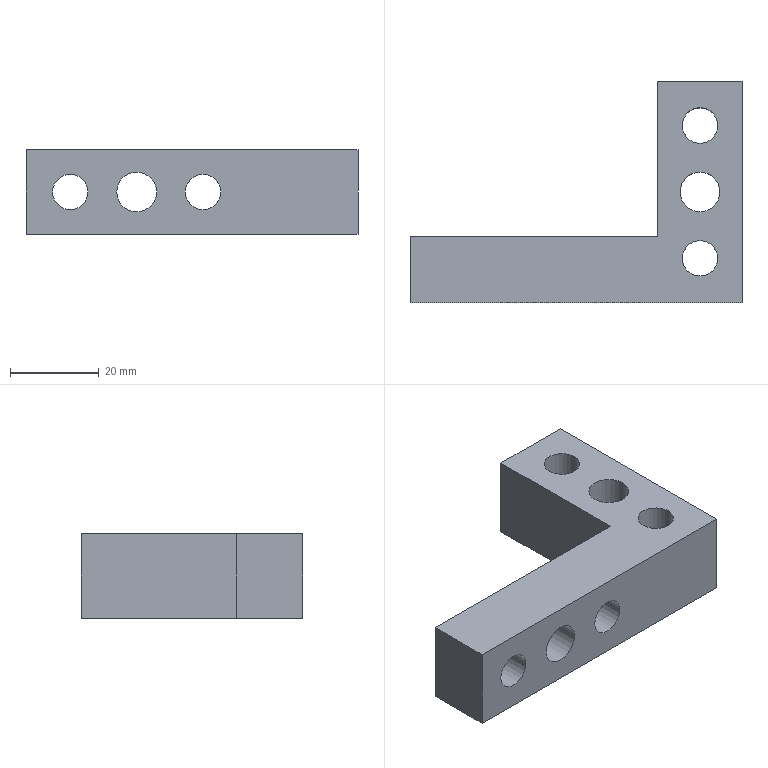Part | SolidWorks | features Extrusion 1, ICE 1 | 1 solid | 20 faces | box 75 x 50 x 19 mm | volume 28429 mm3 | cylinder 12 | plane 8 | commonest cylinder face diameters 8 x8 9 x4
STEP:
#1=CARTESIAN_POINT('',(14.,0.,9.5));
#2=VERTEX_POINT('',#1);
#3=CARTESIAN_POINT('',(6.,0.,9.5));
#4=VERTEX_POINT('',#3);
#5=CARTESIAN_POINT('',(10.,0.,9.5));
#6=DIRECTION('',(0.,1.,0.));
#7=DIRECTION('',(0.,0.,1.));
#8=AXIS2_PLACEMENT_3D('',#5,#6,#7);
#9=CIRCLE('',#8,4.);
#10=EDGE_CURVE('',#2,#4,#9,.T.);
#11=ORIENTED_EDGE('',*,*,#10,.F.);
#12=CARTESIAN_POINT('',(14.,15.,9.5));
#13=VERTEX_POINT('',#12);
#14=CARTESIAN_POINT('',(14.,-4.,9.5));
#15=DIRECTION('',(0.,1.,0.));
#16=VECTOR('',#15,1000.);
#17=LINE('',#14,#16);
#18=EDGE_CURVE('',#2,#13,#17,.T.);
#19=ORIENTED_EDGE('',*,*,#18,.T.);
#20=CARTESIAN_POINT('',(6.,15.,9.5));
#21=VERTEX_POINT('',#20);
#22=CARTESIAN_POINT('',(10.,15.,9.5));
#23=DIRECTION('',(0.,1.,0.));
#24=DIRECTION('',(-1.,0.,0.));
#25=AXIS2_PLACEMENT_3D('',#22,#23,#24);
#26=CIRCLE('',#25,4.);
#27=EDGE_CURVE('',#13,#21,#26,.T.);
#28=ORIENTED_EDGE('',*,*,#27,.T.);
#29=CARTESIAN_POINT('',(6.,-4.,9.5));
#30=DIRECTION('',(0.,1.,0.));
#31=VECTOR('',#30,1000.);
#32=LINE('',#29,#31);
#33=EDGE_CURVE('',#4,#21,#32,.T.);
#34=ORIENTED_EDGE('',*,*,#33,.F.);
#35=EDGE_LOOP('',(#11,#19,#28,#34));
#36=FACE_OUTER_BOUND('',#35,.T.);
#37=CARTESIAN_POINT('',(10.,-4.,9.5));
#38=DIRECTION('',(0.,1.,0.));
#39=DIRECTION('',(-1.,0.,0.));
#40=AXIS2_PLACEMENT_3D('',#37,#38,#39);
#41=CYLINDRICAL_SURFACE('',#40,4.);
#42=ADVANCED_FACE('',(#36),#41,.F.);
#43=CARTESIAN_POINT('',(29.5,0.,9.5));
#44=VERTEX_POINT('',#43);
#45=CARTESIAN_POINT('',(20.5,0.,9.5));
#46=VERTEX_POINT('',#45);
#47=CARTESIAN_POINT('',(25.,0.,9.5));
#48=DIRECTION('',(0.,1.,0.));
#49=DIRECTION('',(0.,0.,1.));
#50=AXIS2_PLACEMENT_3D('',#47,#48,#49);
#51=CIRCLE('',#50,4.5);
#52=EDGE_CURVE('',#44,#46,#51,.T.);
#53=ORIENTED_EDGE('',*,*,#52,.F.);
#54=CARTESIAN_POINT('',(29.5,15.,9.5));
#55=VERTEX_POINT('',#54);
#56=CARTESIAN_POINT('',(29.5,-4.,9.5));
#57=DIRECTION('',(0.,1.,0.));
#58=VECTOR('',#57,1000.);
#59=LINE('',#56,#58);
#60=EDGE_CURVE('',#44,#55,#59,.T.);
#61=ORIENTED_EDGE('',*,*,#60,.T.);
#62=CARTESIAN_POINT('',(20.5,15.,9.5));
#63=VERTEX_POINT('',#62);
#64=CARTESIAN_POINT('',(25.,15.,9.5));
#65=DIRECTION('',(0.,1.,0.));
#66=DIRECTION('',(-1.,0.,0.));
#67=AXIS2_PLACEMENT_3D('',#64,#65,#66);
#68=CIRCLE('',#67,4.5);
#69=EDGE_CURVE('',#55,#63,#68,.T.);
#70=ORIENTED_EDGE('',*,*,#69,.T.);
#71=CARTESIAN_POINT('',(20.5,-4.,9.5));
#72=DIRECTION('',(0.,1.,0.));
#73=VECTOR('',#72,1000.);
#74=LINE('',#71,#73);
#75=EDGE_CURVE('',#46,#63,#74,.T.);
#76=ORIENTED_EDGE('',*,*,#75,.F.);
#77=EDGE_LOOP('',(#53,#61,#70,#76));
#78=FACE_OUTER_BOUND('',#77,.T.);
#79=CARTESIAN_POINT('',(25.,-4.,9.5));
#80=DIRECTION('',(0.,1.,0.));
#81=DIRECTION('',(-1.,0.,0.));
#82=AXIS2_PLACEMENT_3D('',#79,#80,#81);
#83=CYLINDRICAL_SURFACE('',#82,4.5);
#84=ADVANCED_FACE('',(#78),#83,.F.);
#85=CARTESIAN_POINT('',(44.,0.,9.5));
#86=VERTEX_POINT('',#85);
#87=CARTESIAN_POINT('',(36.,0.,9.5));
#88=VERTEX_POINT('',#87);
#89=CARTESIAN_POINT('',(40.,0.,9.5));
#90=DIRECTION('',(0.,1.,0.));
#91=DIRECTION('',(0.,0.,1.));
#92=AXIS2_PLACEMENT_3D('',#89,#90,#91);
#93=CIRCLE('',#92,4.);
#94=EDGE_CURVE('',#86,#88,#93,.T.);
#95=ORIENTED_EDGE('',*,*,#94,.F.);
#96=CARTESIAN_POINT('',(44.,15.,9.5));
#97=VERTEX_POINT('',#96);
#98=CARTESIAN_POINT('',(44.,-4.,9.5));
#99=DIRECTION('',(0.,1.,0.));
#100=VECTOR('',#99,1000.);
#101=LINE('',#98,#100);
#102=EDGE_CURVE('',#86,#97,#101,.T.);
#103=ORIENTED_EDGE('',*,*,#102,.T.);
#104=CARTESIAN_POINT('',(36.,15.,9.5));
#105=VERTEX_POINT('',#104);
#106=CARTESIAN_POINT('',(40.,15.,9.5));
#107=DIRECTION('',(0.,1.,0.));
#108=DIRECTION('',(-1.,0.,0.));
#109=AXIS2_PLACEMENT_3D('',#106,#107,#108);
#110=CIRCLE('',#109,4.);
#111=EDGE_CURVE('',#97,#105,#110,.T.);
#112=ORIENTED_EDGE('',*,*,#111,.T.);
#113=CARTESIAN_POINT('',(36.,-4.,9.5));
#114=DIRECTION('',(0.,1.,0.));
#115=VECTOR('',#114,1000.);
#116=LINE('',#113,#115);
#117=EDGE_CURVE('',#88,#105,#116,.T.);
#118=ORIENTED_EDGE('',*,*,#117,.F.);
#119=EDGE_LOOP('',(#95,#103,#112,#118));
#120=FACE_OUTER_BOUND('',#119,.T.);
#121=CARTESIAN_POINT('',(40.,-4.,9.5));
#122=DIRECTION('',(0.,1.,0.));
#123=DIRECTION('',(-1.,0.,0.));
#124=AXIS2_PLACEMENT_3D('',#121,#122,#123);
#125=CYLINDRICAL_SURFACE('',#124,4.);
#126=ADVANCED_FACE('',(#120),#125,.F.);
#127=CARTESIAN_POINT('',(61.5,40.,19.));
#128=VERTEX_POINT('',#127);
#129=CARTESIAN_POINT('',(69.5,40.,19.));
#130=VERTEX_POINT('',#129);
#131=CARTESIAN_POINT('',(65.5,40.,19.));
#132=DIRECTION('',(0.,0.,1.));
#133=DIRECTION('',(1.,0.,0.));
#134=AXIS2_PLACEMENT_3D('',#131,#132,#133);
#135=CIRCLE('',#134,4.);
#136=EDGE_CURVE('',#128,#130,#135,.T.);
#137=ORIENTED_EDGE('',*,*,#136,.T.);
#138=CARTESIAN_POINT('',(69.5,40.,0.));
#139=VERTEX_POINT('',#138);
#140=CARTESIAN_POINT('',(69.5,40.,19.));
#141=DIRECTION('',(0.,0.,-1.));
#142=VECTOR('',#141,1000.);
#143=LINE('',#140,#142);
#144=EDGE_CURVE('',#130,#139,#143,.T.);
#145=ORIENTED_EDGE('',*,*,#144,.T.);
#146=CARTESIAN_POINT('',(61.5,40.,0.));
#147=VERTEX_POINT('',#146);
#148=CARTESIAN_POINT('',(65.5,40.,0.));
#149=DIRECTION('',(0.,0.,1.));
#150=DIRECTION('',(1.,0.,0.));
#151=AXIS2_PLACEMENT_3D('',#148,#149,#150);
#152=CIRCLE('',#151,4.);
#153=EDGE_CURVE('',#147,#139,#152,.T.);
#154=ORIENTED_EDGE('',*,*,#153,.F.);
#155=CARTESIAN_POINT('',(61.5,40.,19.));
#156=DIRECTION('',(0.,0.,-1.));
#157=VECTOR('',#156,1000.);
#158=LINE('',#155,#157);
#159=EDGE_CURVE('',#128,#147,#158,.T.);
#160=ORIENTED_EDGE('',*,*,#159,.F.);
#161=EDGE_LOOP('',(#137,#145,#154,#160));
#162=FACE_OUTER_BOUND('',#161,.T.);
#163=CARTESIAN_POINT('',(65.5,40.,19.));
#164=DIRECTION('',(0.,0.,-1.));
#165=DIRECTION('',(-1.,0.,0.));
#166=AXIS2_PLACEMENT_3D('',#163,#164,#165);
#167=CYLINDRICAL_SURFACE('',#166,4.);
#168=ADVANCED_FACE('',(#162),#167,.F.);
#169=CARTESIAN_POINT('',(61.,25.,19.));
#170=VERTEX_POINT('',#169);
#171=CARTESIAN_POINT('',(70.,25.,19.));
#172=VERTEX_POINT('',#171);
#173=CARTESIAN_POINT('',(65.5,25.,19.));
#174=DIRECTION('',(0.,0.,1.));
#175=DIRECTION('',(1.,0.,0.));
#176=AXIS2_PLACEMENT_3D('',#173,#174,#175);
#177=CIRCLE('',#176,4.5);
#178=EDGE_CURVE('',#170,#172,#177,.T.);
#179=ORIENTED_EDGE('',*,*,#178,.T.);
#180=CARTESIAN_POINT('',(70.,25.,0.));
#181=VERTEX_POINT('',#180);
#182=CARTESIAN_POINT('',(70.,25.,19.));
#183=DIRECTION('',(0.,0.,-1.));
#184=VECTOR('',#183,1000.);
#185=LINE('',#182,#184);
#186=EDGE_CURVE('',#172,#181,#185,.T.);
#187=ORIENTED_EDGE('',*,*,#186,.T.);
#188=CARTESIAN_POINT('',(61.,25.,0.));
#189=VERTEX_POINT('',#188);
#190=CARTESIAN_POINT('',(65.5,25.,0.));
#191=DIRECTION('',(0.,0.,1.));
#192=DIRECTION('',(1.,0.,0.));
#193=AXIS2_PLACEMENT_3D('',#190,#191,#192);
#194=CIRCLE('',#193,4.5);
#195=EDGE_CURVE('',#189,#181,#194,.T.);
#196=ORIENTED_EDGE('',*,*,#195,.F.);
#197=CARTESIAN_POINT('',(61.,25.,19.));
#198=DIRECTION('',(0.,0.,-1.));
#199=VECTOR('',#198,1000.);
#200=LINE('',#197,#199);
#201=EDGE_CURVE('',#170,#189,#200,.T.);
#202=ORIENTED_EDGE('',*,*,#201,.F.);
#203=EDGE_LOOP('',(#179,#187,#196,#202));
#204=FACE_OUTER_BOUND('',#203,.T.);
#205=CARTESIAN_POINT('',(65.5,25.,19.));
#206=DIRECTION('',(0.,0.,-1.));
#207=DIRECTION('',(-1.,0.,0.));
#208=AXIS2_PLACEMENT_3D('',#205,#206,#207);
#209=CYLINDRICAL_SURFACE('',#208,4.5);
#210=ADVANCED_FACE('',(#204),#209,.F.);
#211=CARTESIAN_POINT('',(61.5,10.,19.));
#212=VERTEX_POINT('',#211);
#213=CARTESIAN_POINT('',(69.5,10.,19.));
#214=VERTEX_POINT('',#213);
#215=CARTESIAN_POINT('',(65.5,10.,19.));
#216=DIRECTION('',(0.,0.,1.));
#217=DIRECTION('',(1.,0.,0.));
#218=AXIS2_PLACEMENT_3D('',#215,#216,#217);
#219=CIRCLE('',#218,4.);
#220=EDGE_CURVE('',#212,#214,#219,.T.);
#221=ORIENTED_EDGE('',*,*,#220,.T.);
#222=CARTESIAN_POINT('',(69.5,10.,0.));
#223=VERTEX_POINT('',#222);
#224=CARTESIAN_POINT('',(69.5,10.,19.));
#225=DIRECTION('',(0.,0.,-1.));
#226=VECTOR('',#225,1000.);
#227=LINE('',#224,#226);
#228=EDGE_CURVE('',#214,#223,#227,.T.);
#229=ORIENTED_EDGE('',*,*,#228,.T.);
#230=CARTESIAN_POINT('',(61.5,10.,0.));
#231=VERTEX_POINT('',#230);
#232=CARTESIAN_POINT('',(65.5,10.,0.));
#233=DIRECTION('',(0.,0.,1.));
#234=DIRECTION('',(1.,0.,0.));
#235=AXIS2_PLACEMENT_3D('',#232,#233,#234);
#236=CIRCLE('',#235,4.);
#237=EDGE_CURVE('',#231,#223,#236,.T.);
#238=ORIENTED_EDGE('',*,*,#237,.F.);
#239=CARTESIAN_POINT('',(61.5,10.,19.));
#240=DIRECTION('',(0.,0.,-1.));
#241=VECTOR('',#240,1000.);
#242=LINE('',#239,#241);
#243=EDGE_CURVE('',#212,#231,#242,.T.);
#244=ORIENTED_EDGE('',*,*,#243,.F.);
#245=EDGE_LOOP('',(#221,#229,#238,#244));
#246=FACE_OUTER_BOUND('',#245,.T.);
#247=CARTESIAN_POINT('',(65.5,10.,19.));
#248=DIRECTION('',(0.,0.,-1.));
#249=DIRECTION('',(-1.,0.,0.));
#250=AXIS2_PLACEMENT_3D('',#247,#248,#249);
#251=CYLINDRICAL_SURFACE('',#250,4.);
#252=ADVANCED_FACE('',(#246),#251,.F.);
#253=ORIENTED_EDGE('',*,*,#178,.F.);
#254=CARTESIAN_POINT('',(65.5,25.,19.));
#255=DIRECTION('',(0.,0.,1.));
#256=DIRECTION('',(1.,0.,0.));
#257=AXIS2_PLACEMENT_3D('',#254,#255,#256);
#258=CIRCLE('',#257,4.5);
#259=EDGE_CURVE('',#172,#170,#258,.T.);
#260=ORIENTED_EDGE('',*,*,#259,.F.);
#261=EDGE_LOOP('',(#253,#260));
#262=FACE_BOUND('',#261,.T.);
#263=CARTESIAN_POINT('',(0.,15.,19.));
#264=VERTEX_POINT('',#263);
#265=CARTESIAN_POINT('',(0.,0.,19.));
#266=VERTEX_POINT('',#265);
#267=CARTESIAN_POINT('',(0.,15.,19.));
#268=DIRECTION('',(0.,-1.,0.));
#269=VECTOR('',#268,1000.);
#270=LINE('',#267,#269);
#271=EDGE_CURVE('',#264,#266,#270,.T.);
#272=ORIENTED_EDGE('',*,*,#271,.T.);
#273=CARTESIAN_POINT('',(75.,0.,19.));
#274=VERTEX_POINT('',#273);
#275=CARTESIAN_POINT('',(0.,0.,19.));
#276=DIRECTION('',(1.,0.,0.));
#277=VECTOR('',#276,1000.);
#278=LINE('',#275,#277);
#279=EDGE_CURVE('',#266,#274,#278,.T.);
#280=ORIENTED_EDGE('',*,*,#279,.T.);
#281=CARTESIAN_POINT('',(75.,50.,19.));
#282=VERTEX_POINT('',#281);
#283=CARTESIAN_POINT('',(75.,0.,19.));
#284=DIRECTION('',(0.,1.,0.));
#285=VECTOR('',#284,1000.);
#286=LINE('',#283,#285);
#287=EDGE_CURVE('',#274,#282,#286,.T.);
#288=ORIENTED_EDGE('',*,*,#287,.T.);
#289=CARTESIAN_POINT('',(56.,50.,19.));
#290=VERTEX_POINT('',#289);
#291=CARTESIAN_POINT('',(75.,50.,19.));
#292=DIRECTION('',(-1.,0.,0.));
#293=VECTOR('',#292,1000.);
#294=LINE('',#291,#293);
#295=EDGE_CURVE('',#282,#290,#294,.T.);
#296=ORIENTED_EDGE('',*,*,#295,.T.);
#297=CARTESIAN_POINT('',(56.,15.,19.));
#298=VERTEX_POINT('',#297);
#299=CARTESIAN_POINT('',(56.,50.,19.));
#300=DIRECTION('',(0.,-1.,0.));
#301=VECTOR('',#300,1000.);
#302=LINE('',#299,#301);
#303=EDGE_CURVE('',#290,#298,#302,.T.);
#304=ORIENTED_EDGE('',*,*,#303,.T.);
#305=CARTESIAN_POINT('',(56.,15.,19.));
#306=DIRECTION('',(-1.,0.,0.));
#307=VECTOR('',#306,1000.);
#308=LINE('',#305,#307);
#309=EDGE_CURVE('',#298,#264,#308,.T.);
#310=ORIENTED_EDGE('',*,*,#309,.T.);
#311=EDGE_LOOP('',(#272,#280,#288,#296,#304,#310));
#312=FACE_OUTER_BOUND('',#311,.T.);
#313=ORIENTED_EDGE('',*,*,#220,.F.);
#314=CARTESIAN_POINT('',(65.5,10.,19.));
#315=DIRECTION('',(0.,0.,1.));
#316=DIRECTION('',(1.,0.,0.));
#317=AXIS2_PLACEMENT_3D('',#314,#315,#316);
#318=CIRCLE('',#317,4.);
#319=EDGE_CURVE('',#214,#212,#318,.T.);
#320=ORIENTED_EDGE('',*,*,#319,.F.);
#321=EDGE_LOOP('',(#313,#320));
#322=FACE_BOUND('',#321,.T.);
#323=ORIENTED_EDGE('',*,*,#136,.F.);
#324=CARTESIAN_POINT('',(65.5,40.,19.));
#325=DIRECTION('',(0.,0.,1.));
#326=DIRECTION('',(1.,0.,0.));
#327=AXIS2_PLACEMENT_3D('',#324,#325,#326);
#328=CIRCLE('',#327,4.);
#329=EDGE_CURVE('',#130,#128,#328,.T.);
#330=ORIENTED_EDGE('',*,*,#329,.F.);
#331=EDGE_LOOP('',(#323,#330));
#332=FACE_BOUND('',#331,.T.);
#333=CARTESIAN_POINT('',(0.,0.,19.));
#334=DIRECTION('',(0.,0.,1.));
#335=DIRECTION('',(1.,0.,0.));
#336=AXIS2_PLACEMENT_3D('',#333,#334,#335);
#337=PLANE('',#336);
#338=ADVANCED_FACE('',(#262,#312,#322,#332),#337,.T.);
#339=CARTESIAN_POINT('',(0.,15.,0.));
#340=VERTEX_POINT('',#339);
#341=CARTESIAN_POINT('',(0.,0.,0.));
#342=VERTEX_POINT('',#341);
#343=CARTESIAN_POINT('',(0.,15.,0.));
#344=DIRECTION('',(0.,-1.,0.));
#345=VECTOR('',#344,1000.);
#346=LINE('',#343,#345);
#347=EDGE_CURVE('',#340,#342,#346,.T.);
#348=ORIENTED_EDGE('',*,*,#347,.F.);
#349=CARTESIAN_POINT('',(56.,15.,0.));
#350=VERTEX_POINT('',#349);
#351=CARTESIAN_POINT('',(56.,15.,0.));
#352=DIRECTION('',(-1.,0.,0.));
#353=VECTOR('',#352,1000.);
#354=LINE('',#351,#353);
#355=EDGE_CURVE('',#350,#340,#354,.T.);
#356=ORIENTED_EDGE('',*,*,#355,.F.);
#357=CARTESIAN_POINT('',(56.,50.,0.));
#358=VERTEX_POINT('',#357);
#359=CARTESIAN_POINT('',(56.,50.,0.));
#360=DIRECTION('',(0.,-1.,0.));
#361=VECTOR('',#360,1000.);
#362=LINE('',#359,#361);
#363=EDGE_CURVE('',#358,#350,#362,.T.);
#364=ORIENTED_EDGE('',*,*,#363,.F.);
#365=CARTESIAN_POINT('',(75.,50.,0.));
#366=VERTEX_POINT('',#365);
#367=CARTESIAN_POINT('',(75.,50.,0.));
#368=DIRECTION('',(-1.,0.,0.));
#369=VECTOR('',#368,1000.);
#370=LINE('',#367,#369);
#371=EDGE_CURVE('',#366,#358,#370,.T.);
#372=ORIENTED_EDGE('',*,*,#371,.F.);
#373=CARTESIAN_POINT('',(75.,0.,0.));
#374=VERTEX_POINT('',#373);
#375=CARTESIAN_POINT('',(75.,0.,0.));
#376=DIRECTION('',(0.,1.,0.));
#377=VECTOR('',#376,1000.);
#378=LINE('',#375,#377);
#379=EDGE_CURVE('',#374,#366,#378,.T.);
#380=ORIENTED_EDGE('',*,*,#379,.F.);
#381=CARTESIAN_POINT('',(0.,0.,0.));
#382=DIRECTION('',(1.,0.,0.));
#383=VECTOR('',#382,1000.);
#384=LINE('',#381,#383);
#385=EDGE_CURVE('',#342,#374,#384,.T.);
#386=ORIENTED_EDGE('',*,*,#385,.F.);
#387=EDGE_LOOP('',(#348,#356,#364,#372,#380,#386));
#388=FACE_OUTER_BOUND('',#387,.T.);
#389=ORIENTED_EDGE('',*,*,#237,.T.);
#390=CARTESIAN_POINT('',(65.5,10.,0.));
#391=DIRECTION('',(0.,0.,1.));
#392=DIRECTION('',(1.,0.,0.));
#393=AXIS2_PLACEMENT_3D('',#390,#391,#392);
#394=CIRCLE('',#393,4.);
#395=EDGE_CURVE('',#223,#231,#394,.T.);
#396=ORIENTED_EDGE('',*,*,#395,.T.);
#397=EDGE_LOOP('',(#389,#396));
#398=FACE_BOUND('',#397,.T.);
#399=ORIENTED_EDGE('',*,*,#195,.T.);
#400=CARTESIAN_POINT('',(65.5,25.,0.));
#401=DIRECTION('',(0.,0.,1.));
#402=DIRECTION('',(1.,0.,0.));
#403=AXIS2_PLACEMENT_3D('',#400,#401,#402);
#404=CIRCLE('',#403,4.5);
#405=EDGE_CURVE('',#181,#189,#404,.T.);
#406=ORIENTED_EDGE('',*,*,#405,.T.);
#407=EDGE_LOOP('',(#399,#406));
#408=FACE_BOUND('',#407,.T.);
#409=ORIENTED_EDGE('',*,*,#153,.T.);
#410=CARTESIAN_POINT('',(65.5,40.,0.));
#411=DIRECTION('',(0.,0.,1.));
#412=DIRECTION('',(1.,0.,0.));
#413=AXIS2_PLACEMENT_3D('',#410,#411,#412);
#414=CIRCLE('',#413,4.);
#415=EDGE_CURVE('',#139,#147,#414,.T.);
#416=ORIENTED_EDGE('',*,*,#415,.T.);
#417=EDGE_LOOP('',(#409,#416));
#418=FACE_BOUND('',#417,.T.);
#419=CARTESIAN_POINT('',(0.,0.,0.));
#420=DIRECTION('',(0.,0.,1.));
#421=DIRECTION('',(1.,0.,0.));
#422=AXIS2_PLACEMENT_3D('',#419,#420,#421);
#423=PLANE('',#422);
#424=ADVANCED_FACE('',(#388,#398,#408,#418),#423,.F.);
#425=ORIENTED_EDGE('',*,*,#347,.T.);
#426=CARTESIAN_POINT('',(0.,0.,19.));
#427=DIRECTION('',(0.,0.,-1.));
#428=VECTOR('',#427,1000.);
#429=LINE('',#426,#428);
#430=EDGE_CURVE('',#266,#342,#429,.T.);
#431=ORIENTED_EDGE('',*,*,#430,.F.);
#432=ORIENTED_EDGE('',*,*,#271,.F.);
#433=CARTESIAN_POINT('',(0.,15.,19.));
#434=DIRECTION('',(0.,0.,-1.));
#435=VECTOR('',#434,1000.);
#436=LINE('',#433,#435);
#437=EDGE_CURVE('',#264,#340,#436,.T.);
#438=ORIENTED_EDGE('',*,*,#437,.T.);
#439=EDGE_LOOP('',(#425,#431,#432,#438));
#440=FACE_OUTER_BOUND('',#439,.T.);
#441=CARTESIAN_POINT('',(0.,15.,19.));
#442=DIRECTION('',(1.,0.,0.));
#443=DIRECTION('',(0.,1.,0.));
#444=AXIS2_PLACEMENT_3D('',#441,#442,#443);
#445=PLANE('',#444);
#446=ADVANCED_FACE('',(#440),#445,.F.);
#447=CARTESIAN_POINT('',(10.,0.,9.5));
#448=DIRECTION('',(0.,1.,0.));
#449=DIRECTION('',(0.,0.,1.));
#450=AXIS2_PLACEMENT_3D('',#447,#448,#449);
#451=CIRCLE('',#450,4.);
#452=EDGE_CURVE('',#4,#2,#451,.T.);
#453=ORIENTED_EDGE('',*,*,#452,.T.);
#454=ORIENTED_EDGE('',*,*,#10,.T.);
#455=EDGE_LOOP('',(#453,#454));
#456=FACE_BOUND('',#455,.T.);
#457=CARTESIAN_POINT('',(25.,0.,9.5));
#458=DIRECTION('',(0.,1.,0.));
#459=DIRECTION('',(0.,0.,1.));
#460=AXIS2_PLACEMENT_3D('',#457,#458,#459);
#461=CIRCLE('',#460,4.5);
#462=EDGE_CURVE('',#46,#44,#461,.T.);
#463=ORIENTED_EDGE('',*,*,#462,.T.);
#464=ORIENTED_EDGE('',*,*,#52,.T.);
#465=EDGE_LOOP('',(#463,#464));
#466=FACE_BOUND('',#465,.T.);
#467=CARTESIAN_POINT('',(40.,0.,9.5));
#468=DIRECTION('',(0.,1.,0.));
#469=DIRECTION('',(0.,0.,1.));
#470=AXIS2_PLACEMENT_3D('',#467,#468,#469);
#471=CIRCLE('',#470,4.);
#472=EDGE_CURVE('',#88,#86,#471,.T.);
#473=ORIENTED_EDGE('',*,*,#472,.T.);
#474=ORIENTED_EDGE('',*,*,#94,.T.);
#475=EDGE_LOOP('',(#473,#474));
#476=FACE_BOUND('',#475,.T.);
#477=ORIENTED_EDGE('',*,*,#385,.T.);
#478=CARTESIAN_POINT('',(75.,0.,19.));
#479=DIRECTION('',(0.,0.,-1.));
#480=VECTOR('',#479,1000.);
#481=LINE('',#478,#480);
#482=EDGE_CURVE('',#274,#374,#481,.T.);
#483=ORIENTED_EDGE('',*,*,#482,.F.);
#484=ORIENTED_EDGE('',*,*,#279,.F.);
#485=ORIENTED_EDGE('',*,*,#430,.T.);
#486=EDGE_LOOP('',(#477,#483,#484,#485));
#487=FACE_OUTER_BOUND('',#486,.T.);
#488=CARTESIAN_POINT('',(0.,0.,19.));
#489=DIRECTION('',(0.,1.,0.));
#490=DIRECTION('',(0.,0.,1.));
#491=AXIS2_PLACEMENT_3D('',#488,#489,#490);
#492=PLANE('',#491);
#493=ADVANCED_FACE('',(#456,#466,#476,#487),#492,.F.);
#494=ORIENTED_EDGE('',*,*,#379,.T.);
#495=CARTESIAN_POINT('',(75.,50.,19.));
#496=DIRECTION('',(0.,0.,-1.));
#497=VECTOR('',#496,1000.);
#498=LINE('',#495,#497);
#499=EDGE_CURVE('',#282,#366,#498,.T.);
#500=ORIENTED_EDGE('',*,*,#499,.F.);
#501=ORIENTED_EDGE('',*,*,#287,.F.);
#502=ORIENTED_EDGE('',*,*,#482,.T.);
#503=EDGE_LOOP('',(#494,#500,#501,#502));
#504=FACE_OUTER_BOUND('',#503,.T.);
#505=CARTESIAN_POINT('',(75.,0.,19.));
#506=DIRECTION('',(-1.,0.,0.));
#507=DIRECTION('',(0.,0.,1.));
#508=AXIS2_PLACEMENT_3D('',#505,#506,#507);
#509=PLANE('',#508);
#510=ADVANCED_FACE('',(#504),#509,.F.);
#511=ORIENTED_EDGE('',*,*,#371,.T.);
#512=CARTESIAN_POINT('',(56.,50.,19.));
#513=DIRECTION('',(0.,0.,-1.));
#514=VECTOR('',#513,1000.);
#515=LINE('',#512,#514);
#516=EDGE_CURVE('',#290,#358,#515,.T.);
#517=ORIENTED_EDGE('',*,*,#516,.F.);
#518=ORIENTED_EDGE('',*,*,#295,.F.);
#519=ORIENTED_EDGE('',*,*,#499,.T.);
#520=EDGE_LOOP('',(#511,#517,#518,#519));
#521=FACE_OUTER_BOUND('',#520,.T.);
#522=CARTESIAN_POINT('',(75.,50.,19.));
#523=DIRECTION('',(0.,-1.,0.));
#524=DIRECTION('',(0.,0.,-1.));
#525=AXIS2_PLACEMENT_3D('',#522,#523,#524);
#526=PLANE('',#525);
#527=ADVANCED_FACE('',(#521),#526,.F.);
#528=ORIENTED_EDGE('',*,*,#363,.T.);
#529=CARTESIAN_POINT('',(56.,15.,19.));
#530=DIRECTION('',(0.,0.,-1.));
#531=VECTOR('',#530,1000.);
#532=LINE('',#529,#531);
#533=EDGE_CURVE('',#298,#350,#532,.T.);
#534=ORIENTED_EDGE('',*,*,#533,.F.);
#535=ORIENTED_EDGE('',*,*,#303,.F.);
#536=ORIENTED_EDGE('',*,*,#516,.T.);
#537=EDGE_LOOP('',(#528,#534,#535,#536));
#538=FACE_OUTER_BOUND('',#537,.T.);
#539=CARTESIAN_POINT('',(56.,50.,19.));
#540=DIRECTION('',(1.,0.,0.));
#541=DIRECTION('',(0.,1.,0.));
#542=AXIS2_PLACEMENT_3D('',#539,#540,#541);
#543=PLANE('',#542);
#544=ADVANCED_FACE('',(#538),#543,.F.);
#545=CARTESIAN_POINT('',(10.,15.,9.5));
#546=DIRECTION('',(0.,1.,0.));
#547=DIRECTION('',(-1.,0.,0.));
#548=AXIS2_PLACEMENT_3D('',#545,#546,#547);
#549=CIRCLE('',#548,4.);
#550=EDGE_CURVE('',#21,#13,#549,.T.);
#551=ORIENTED_EDGE('',*,*,#550,.F.);
#552=ORIENTED_EDGE('',*,*,#27,.F.);
#553=EDGE_LOOP('',(#551,#552));
#554=FACE_BOUND('',#553,.T.);
#555=CARTESIAN_POINT('',(25.,15.,9.5));
#556=DIRECTION('',(0.,1.,0.));
#557=DIRECTION('',(-1.,0.,0.));
#558=AXIS2_PLACEMENT_3D('',#555,#556,#557);
#559=CIRCLE('',#558,4.5);
#560=EDGE_CURVE('',#63,#55,#559,.T.);
#561=ORIENTED_EDGE('',*,*,#560,.F.);
#562=ORIENTED_EDGE('',*,*,#69,.F.);
#563=EDGE_LOOP('',(#561,#562));
#564=FACE_BOUND('',#563,.T.);
#565=CARTESIAN_POINT('',(40.,15.,9.5));
#566=DIRECTION('',(0.,1.,0.));
#567=DIRECTION('',(-1.,0.,0.));
#568=AXIS2_PLACEMENT_3D('',#565,#566,#567);
#569=CIRCLE('',#568,4.);
#570=EDGE_CURVE('',#105,#97,#569,.T.);
#571=ORIENTED_EDGE('',*,*,#570,.F.);
#572=ORIENTED_EDGE('',*,*,#111,.F.);
#573=EDGE_LOOP('',(#571,#572));
#574=FACE_BOUND('',#573,.T.);
#575=ORIENTED_EDGE('',*,*,#355,.T.);
#576=ORIENTED_EDGE('',*,*,#437,.F.);
#577=ORIENTED_EDGE('',*,*,#309,.F.);
#578=ORIENTED_EDGE('',*,*,#533,.T.);
#579=EDGE_LOOP('',(#575,#576,#577,#578));
#580=FACE_OUTER_BOUND('',#579,.T.);
#581=CARTESIAN_POINT('',(56.,15.,19.));
#582=DIRECTION('',(0.,-1.,0.));
#583=DIRECTION('',(1.,0.,0.));
#584=AXIS2_PLACEMENT_3D('',#581,#582,#583);
#585=PLANE('',#584);
#586=ADVANCED_FACE('',(#554,#564,#574,#580),#585,.F.);
#587=ORIENTED_EDGE('',*,*,#228,.F.);
#588=ORIENTED_EDGE('',*,*,#319,.T.);
#589=ORIENTED_EDGE('',*,*,#243,.T.);
#590=ORIENTED_EDGE('',*,*,#395,.F.);
#591=EDGE_LOOP('',(#587,#588,#589,#590));
#592=FACE_OUTER_BOUND('',#591,.T.);
#593=CARTESIAN_POINT('',(65.5,10.,19.));
#594=DIRECTION('',(0.,0.,-1.));
#595=DIRECTION('',(-1.,0.,0.));
#596=AXIS2_PLACEMENT_3D('',#593,#594,#595);
#597=CYLINDRICAL_SURFACE('',#596,4.);
#598=ADVANCED_FACE('',(#592),#597,.F.);
#599=ORIENTED_EDGE('',*,*,#186,.F.);
#600=ORIENTED_EDGE('',*,*,#259,.T.);
#601=ORIENTED_EDGE('',*,*,#201,.T.);
#602=ORIENTED_EDGE('',*,*,#405,.F.);
#603=EDGE_LOOP('',(#599,#600,#601,#602));
#604=FACE_OUTER_BOUND('',#603,.T.);
#605=CARTESIAN_POINT('',(65.5,25.,19.));
#606=DIRECTION('',(0.,0.,-1.));
#607=DIRECTION('',(-1.,0.,0.));
#608=AXIS2_PLACEMENT_3D('',#605,#606,#607);
#609=CYLINDRICAL_SURFACE('',#608,4.5);
#610=ADVANCED_FACE('',(#604),#609,.F.);
#611=ORIENTED_EDGE('',*,*,#144,.F.);
#612=ORIENTED_EDGE('',*,*,#329,.T.);
#613=ORIENTED_EDGE('',*,*,#159,.T.);
#614=ORIENTED_EDGE('',*,*,#415,.F.);
#615=EDGE_LOOP('',(#611,#612,#613,#614));
#616=FACE_OUTER_BOUND('',#615,.T.);
#617=CARTESIAN_POINT('',(65.5,40.,19.));
#618=DIRECTION('',(0.,0.,-1.));
#619=DIRECTION('',(-1.,0.,0.));
#620=AXIS2_PLACEMENT_3D('',#617,#618,#619);
#621=CYLINDRICAL_SURFACE('',#620,4.);
#622=ADVANCED_FACE('',(#616),#621,.F.);
#623=ORIENTED_EDGE('',*,*,#102,.F.);
#624=ORIENTED_EDGE('',*,*,#472,.F.);
#625=ORIENTED_EDGE('',*,*,#117,.T.);
#626=ORIENTED_EDGE('',*,*,#570,.T.);
#627=EDGE_LOOP('',(#623,#624,#625,#626));
#628=FACE_OUTER_BOUND('',#627,.T.);
#629=CARTESIAN_POINT('',(40.,-4.,9.5));
#630=DIRECTION('',(0.,1.,0.));
#631=DIRECTION('',(-1.,0.,0.));
#632=AXIS2_PLACEMENT_3D('',#629,#630,#631);
#633=CYLINDRICAL_SURFACE('',#632,4.);
#634=ADVANCED_FACE('',(#628),#633,.F.);
#635=ORIENTED_EDGE('',*,*,#60,.F.);
#636=ORIENTED_EDGE('',*,*,#462,.F.);
#637=ORIENTED_EDGE('',*,*,#75,.T.);
#638=ORIENTED_EDGE('',*,*,#560,.T.);
#639=EDGE_LOOP('',(#635,#636,#637,#638));
#640=FACE_OUTER_BOUND('',#639,.T.);
#641=CARTESIAN_POINT('',(25.,-4.,9.5));
#642=DIRECTION('',(0.,1.,0.));
#643=DIRECTION('',(-1.,0.,0.));
#644=AXIS2_PLACEMENT_3D('',#641,#642,#643);
#645=CYLINDRICAL_SURFACE('',#644,4.5);
#646=ADVANCED_FACE('',(#640),#645,.F.);
#647=ORIENTED_EDGE('',*,*,#18,.F.);
#648=ORIENTED_EDGE('',*,*,#452,.F.);
#649=ORIENTED_EDGE('',*,*,#33,.T.);
#650=ORIENTED_EDGE('',*,*,#550,.T.);
#651=EDGE_LOOP('',(#647,#648,#649,#650));
#652=FACE_OUTER_BOUND('',#651,.T.);
#653=CARTESIAN_POINT('',(10.,-4.,9.5));
#654=DIRECTION('',(0.,1.,0.));
#655=DIRECTION('',(-1.,0.,0.));
#656=AXIS2_PLACEMENT_3D('',#653,#654,#655);
#657=CYLINDRICAL_SURFACE('',#656,4.);
#658=ADVANCED_FACE('',(#652),#657,.F.);
#659=CLOSED_SHELL('',(#42,#84,#126,#168,#210,#252,#338,#424,#446,#493,#510,#527,#544,#586,#598,#610,#622,#634,#646,#658));
#660=MANIFOLD_SOLID_BREP('',#659);
#661=CARTESIAN_POINT('',(0.,0.,0.));
#662=DIRECTION('',(0.,0.,1.));
#663=DIRECTION('',(1.,0.,0.));
#664=AXIS2_PLACEMENT_3D('',#661,#662,#663);
#665=(LENGTH_UNIT()NAMED_UNIT(*)SI_UNIT(.MILLI.,.METRE.));
#666=UNCERTAINTY_MEASURE_WITH_UNIT(LENGTH_MEASURE(0.00001),#665,'','');
#667=(NAMED_UNIT(*)PLANE_ANGLE_UNIT()SI_UNIT($,.RADIAN.));
#668=(NAMED_UNIT(*)SI_UNIT($,.STERADIAN.)SOLID_ANGLE_UNIT());
#669=(GEOMETRIC_REPRESENTATION_CONTEXT(3)GLOBAL_UNCERTAINTY_ASSIGNED_CONTEXT((#666))GLOBAL_UNIT_ASSIGNED_CONTEXT((#665,#667,#668))REPRESENTATION_CONTEXT('',''));
#670=ADVANCED_BREP_SHAPE_REPRESENTATION('',(#660,#664),#669);